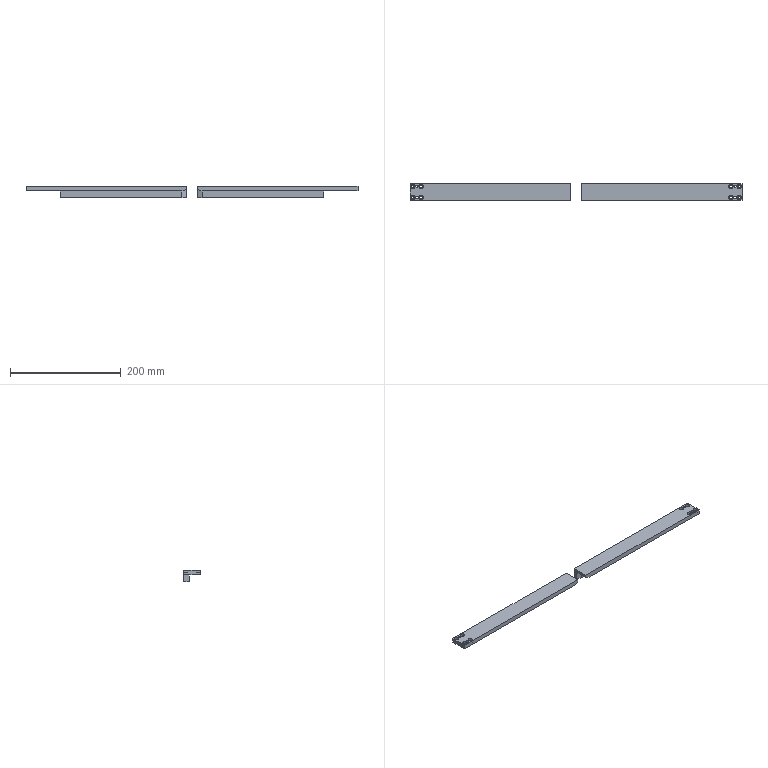NC program | NX | posted with a generic post | part box 600 x 30 x 20 mm
Lines 2675 to 3385 of 3385:
(ZLEVEL_PROFILE_COPY_1_COPY_COPY_COPY_COPY_2_COPY_1 , TOOL : D6A45)
N5306 T02 M6
N5308 G54
N5310 G17 G0 G90 X126.439 Y11.149 S7000 M3
N5312 G43 Z30. H2
N5314 Z-1.
N5316 G94 G1 X125.52 Y12.741 F1000.
N5318 G3 X125. Y13.041 R0.6
N5320 X121.959 Y10. R3.041
N5322 X125. Y13.041 R-3.041
N5324 X124.48 Y12.741 R0.6
N5326 G1 X123.561 Y11.149
N5328 G0 Z30.
N5330 X141.439
N5332 Z-1.
N5334 G1 X140.52 Y12.741
N5336 G3 X140. Y13.041 R0.6
N5338 X136.959 Y10. R3.041
N5340 X140. Y13.041 R-3.041
N5342 X139.48 Y12.741 R0.6
N5344 G1 X138.561 Y11.149
N5346 G0 Z30.
N5348 X133.541 Y-10.5
N5350 Z1.
N5352 G1 Z-1.
N5354 Y-9.5
N5356 G3 X132.5 Y-8.459 R1.041
N5358 X131.459 Y-9.5 R1.041
N5360 G1 Y-10.5
N5362 G3 X132.5 Y-11.541 R1.041
N5364 X133.541 Y-10.5 R1.041
N5366 X133.241 Y-9.98 R0.6
N5368 G0 Z30.
N5370 X123.561 Y-11.149
N5372 Z-1.
N5374 G1 X124.48 Y-12.741
N5376 G3 X125. Y-13.041 R0.6
N5378 X128.041 Y-10. R3.041
N5380 X125. Y-13.041 R-3.041
N5382 X125.52 Y-12.741 R0.6
N5384 G1 X126.439 Y-11.149
N5386 G0 Z30.
N5388 X138.561
N5390 Z-1.
N5392 G1 X139.48 Y-12.741
N5394 G3 X140. Y-13.041 R0.6
N5396 X143.041 Y-10. R3.041
N5398 X140. Y-13.041 R-3.041
N5400 X140.52 Y-12.741 R0.6
N5402 G1 X141.439 Y-11.149
N5404 G0 Z30.
N5406 X132.5 Y11.041
N5408 Z1.
N5410 G1 Z-1.
N5412 G3 X131.459 Y10. R1.041
N5414 X132.5 Y11.041 R-1.041
N5416 X131.98 Y10.741 R0.6
N5418 G0 Z30.
N5420 X-145.92 Y16.95
N5422 Z-1.
N5424 G1 X-145.521 Y16.259
N5426 G3 X-145.001 Y15.959 R0.6
N5428 G1 X145.001
N5430 G2 X145.959 Y15.001 R0.966
N5432 G1 Y-15.001
N5434 G2 X145.001 Y-15.959 R0.966
N5436 G1 X-145.001
N5438 G2 X-145.959 Y-15.001 R0.966
N5440 G1 Y15.001
N5442 G2 X-145.001 Y15.959 R0.966
N5444 G3 X-144.484 Y16.263 R0.6
N5446 G1 X-143.976 Y17.159
N5448 G0 Z30.
N5450 M5
(COMPTOOL10_COPY_1 , TOOL : D3)
N5452 T20 M6
N5454 G54
N5456 G17 G0 G90 X132.456 Y10.143 S7000 M3
N5458 G43 Z30. H20
N5460 Z-0.5
N5462 G94 G1 Z-1. F1000.
N5464 G41 X132.384 Y10.38 D20
N5466 G3 X132.119 Y10.239 R0.3
N5468 G1 X132.116 Y10.235 F850.
N5470 G3 X132.255 Y10.378 R-0.45
N5472 G1 X132.197 Y10.346
N5474 X132.15 Y10.298
N5476 X132.119 Y10.239
N5478 X132.098 Y10.185 Z-1.028
N5480 X132.078 Y10.131 Z-1.056
N5482 X132.063 Y10.075 Z-1.083
N5484 X132.058 Y10.016 Z-1.111
N5486 X132.06 Y9.958 Z-1.139
N5488 X132.068 Y9.9 Z-1.167
N5490 X132.085 Y9.845 Z-1.194
N5492 X132.102 Y9.79 Z-1.222
N5494 X132.138 Y9.744 Z-1.25
N5496 X132.175 Y9.699 Z-1.278
N5498 X132.218 Y9.66 Z-1.306
N5500 X132.265 Y9.625 Z-1.333
N5502 X132.316 Y9.598 Z-1.361
N5504 X132.37 Y9.577 Z-1.389
N5506 X132.426 Y9.564 Z-1.417
N5508 X132.484 Y9.558 Z-1.444
N5510 X132.542 Y9.56 Z-1.472
N5512 X132.599 Y9.568 Z-1.5
N5514 X132.654 Y9.585 Z-1.528
N5516 X132.707 Y9.609 Z-1.556
N5518 X132.757 Y9.64 Z-1.583
N5520 X132.801 Y9.676 Z-1.611
N5522 X132.84 Y9.718 Z-1.639
N5524 X132.875 Y9.765 Z-1.667
N5526 X132.902 Y9.816 Z-1.694
N5528 X132.923 Y9.87 Z-1.722
N5530 X132.936 Y9.926 Z-1.75
N5532 X132.942 Y9.984 Z-1.778
N5534 X132.94 Y10.042 Z-1.806
N5536 X132.932 Y10.099 Z-1.833
N5538 X132.915 Y10.154 Z-1.861
N5540 X132.891 Y10.207 Z-1.889
N5542 X132.86 Y10.257 Z-1.917
N5544 X132.824 Y10.302 Z-1.944
N5546 X132.781 Y10.341 Z-1.972
N5548 X132.739 Y10.381 Z-2.
N5550 X132.735 Y10.384
N5552 G3 X132.255 Y10.378 R0.45
N5554 G1 X132.197 Y10.346
N5556 X132.15 Y10.298
N5558 X132.119 Y10.239
N5560 X132.098 Y10.185 Z-2.028
N5562 X132.078 Y10.131 Z-2.056
N5564 X132.063 Y10.075 Z-2.083
N5566 X132.058 Y10.016 Z-2.111
N5568 X132.06 Y9.958 Z-2.139
N5570 X132.068 Y9.9 Z-2.167
N5572 X132.085 Y9.845 Z-2.194
N5574 X132.102 Y9.79 Z-2.222
N5576 X132.139 Y9.744 Z-2.25
N5578 X132.175 Y9.699 Z-2.278
N5580 X132.218 Y9.66 Z-2.306
N5582 X132.265 Y9.625 Z-2.333
N5584 X132.316 Y9.598 Z-2.361
N5586 X132.37 Y9.577 Z-2.389
N5588 X132.426 Y9.564 Z-2.417
N5590 X132.484 Y9.558 Z-2.444
N5592 X132.542 Y9.56 Z-2.472
N5594 X132.599 Y9.568 Z-2.5
N5596 X132.654 Y9.585 Z-2.528
N5598 X132.707 Y9.609 Z-2.556
N5600 X132.757 Y9.64 Z-2.583
N5602 X132.801 Y9.676 Z-2.611
N5604 X132.84 Y9.718 Z-2.639
N5606 X132.875 Y9.765 Z-2.667
N5608 X132.902 Y9.816 Z-2.694
N5610 X132.923 Y9.87 Z-2.722
N5612 X132.937 Y9.925 Z-2.75
N5614 X132.942 Y9.984 Z-2.778
N5616 X132.94 Y10.042 Z-2.806
N5618 X132.932 Y10.099 Z-2.833
N5620 X132.915 Y10.154 Z-2.861
N5622 X132.891 Y10.207 Z-2.889
N5624 X132.86 Y10.257 Z-2.917
N5626 X132.824 Y10.302 Z-2.944
N5628 X132.781 Y10.341 Z-2.972
N5630 X132.739 Y10.381 Z-3.
N5632 X132.735 Y10.384
N5634 G3 X132.255 Y10.378 R0.45
N5636 G1 X132.197 Y10.346
N5638 X132.15 Y10.298
N5640 X132.119 Y10.239
N5642 X132.098 Y10.185 Z-3.028
N5644 X132.078 Y10.131 Z-3.056
N5646 X132.063 Y10.075 Z-3.083
N5648 X132.058 Y10.016 Z-3.111
N5650 X132.06 Y9.958 Z-3.139
N5652 X132.068 Y9.9 Z-3.167
N5654 X132.085 Y9.845 Z-3.194
N5656 X132.102 Y9.79 Z-3.222
N5658 X132.139 Y9.744 Z-3.25
N5660 X132.175 Y9.699 Z-3.278
N5662 X132.218 Y9.66 Z-3.306
N5664 X132.265 Y9.625 Z-3.333
N5666 X132.316 Y9.598 Z-3.361
N5668 X132.37 Y9.577 Z-3.389
N5670 X132.425 Y9.563 Z-3.417
N5672 X132.484 Y9.558 Z-3.444
N5674 X132.542 Y9.56 Z-3.472
N5676 X132.599 Y9.568 Z-3.5
N5678 X132.654 Y9.585 Z-3.528
N5680 X132.707 Y9.609 Z-3.556
N5682 X132.757 Y9.64 Z-3.583
N5684 X132.801 Y9.676 Z-3.611
N5686 X132.84 Y9.718 Z-3.639
N5688 X132.875 Y9.765 Z-3.667
N5690 X132.902 Y9.816 Z-3.694
N5692 X132.923 Y9.87 Z-3.722
N5694 X132.937 Y9.925 Z-3.75
N5696 X132.942 Y9.984 Z-3.778
N5698 X132.94 Y10.042 Z-3.806
N5700 X132.932 Y10.099 Z-3.833
N5702 X132.915 Y10.154 Z-3.861
N5704 X132.891 Y10.207 Z-3.889
N5706 X132.86 Y10.257 Z-3.917
N5708 X132.824 Y10.302 Z-3.944
N5710 X132.781 Y10.341 Z-3.972
N5712 X132.739 Y10.381 Z-4.
N5714 X132.735 Y10.384
N5716 G3 X132.255 Y10.378 R0.45
N5718 G1 X132.197 Y10.346
N5720 X132.15 Y10.298
N5722 X132.119 Y10.239
N5724 X132.098 Y10.185 Z-4.028
N5726 X132.078 Y10.131 Z-4.056
N5728 X132.063 Y10.075 Z-4.083
N5730 X132.058 Y10.016 Z-4.111
N5732 X132.06 Y9.958 Z-4.139
N5734 X132.068 Y9.9 Z-4.167
N5736 X132.085 Y9.845 Z-4.194
N5738 X132.102 Y9.79 Z-4.222
N5740 X132.139 Y9.744 Z-4.25
N5742 X132.175 Y9.699 Z-4.278
N5744 X132.218 Y9.66 Z-4.306
N5746 X132.265 Y9.625 Z-4.333
N5748 X132.316 Y9.598 Z-4.361
N5750 X132.37 Y9.577 Z-4.389
N5752 X132.425 Y9.563 Z-4.417
N5754 X132.484 Y9.558 Z-4.444
N5756 X132.542 Y9.56 Z-4.472
N5758 X132.599 Y9.568 Z-4.5
N5760 X132.654 Y9.585 Z-4.528
N5762 X132.707 Y9.609 Z-4.556
N5764 X132.757 Y9.64 Z-4.583
N5766 X132.801 Y9.676 Z-4.611
N5768 X132.84 Y9.718 Z-4.639
N5770 X132.875 Y9.765 Z-4.667
N5772 X132.902 Y9.816 Z-4.694
N5774 X132.923 Y9.87 Z-4.722
N5776 X132.937 Y9.925 Z-4.75
N5778 X132.942 Y9.984 Z-4.778
N5780 X132.94 Y10.042 Z-4.806
N5782 X132.932 Y10.099 Z-4.833
N5784 X132.915 Y10.154 Z-4.861
N5786 X132.891 Y10.207 Z-4.889
N5788 X132.86 Y10.257 Z-4.917
N5790 X132.824 Y10.302 Z-4.944
N5792 X132.781 Y10.341 Z-4.972
N5794 X132.739 Y10.381 Z-5.
N5796 X132.735 Y10.384
N5798 G3 X132.255 Y10.378 R0.45
N5800 G1 X132.197 Y10.346
N5802 X132.15 Y10.298
N5804 X132.119 Y10.239
N5806 X132.098 Y10.185 Z-5.028
N5808 X132.078 Y10.131 Z-5.056
N5810 X132.063 Y10.075 Z-5.083
N5812 X132.058 Y10.016 Z-5.111
N5814 X132.06 Y9.958 Z-5.139
N5816 X132.068 Y9.9 Z-5.167
N5818 X132.085 Y9.845 Z-5.194
N5820 X132.102 Y9.79 Z-5.222
N5822 X132.139 Y9.744 Z-5.25
N5824 X132.175 Y9.699 Z-5.278
N5826 X132.218 Y9.66 Z-5.306
N5828 X132.265 Y9.625 Z-5.333
N5830 X132.316 Y9.598 Z-5.361
N5832 X132.37 Y9.577 Z-5.389
N5834 X132.425 Y9.563 Z-5.417
N5836 X132.484 Y9.558 Z-5.444
N5838 X132.542 Y9.56 Z-5.472
N5840 X132.599 Y9.568 Z-5.5
N5842 X132.654 Y9.585 Z-5.528
N5844 X132.707 Y9.609 Z-5.556
N5846 X132.757 Y9.64 Z-5.583
N5848 X132.801 Y9.676 Z-5.611
N5850 X132.84 Y9.718 Z-5.639
N5852 X132.875 Y9.765 Z-5.667
N5854 X132.902 Y9.816 Z-5.694
N5856 X132.923 Y9.87 Z-5.722
N5858 X132.937 Y9.925 Z-5.75
N5860 X132.942 Y9.984 Z-5.778
N5862 X132.94 Y10.042 Z-5.806
N5864 X132.932 Y10.099 Z-5.833
N5866 X132.915 Y10.154 Z-5.861
N5868 X132.891 Y10.207 Z-5.889
N5870 X132.86 Y10.257 Z-5.917
N5872 X132.824 Y10.302 Z-5.944
N5874 X132.781 Y10.341 Z-5.972
N5876 X132.739 Y10.381 Z-6.
N5878 X132.735 Y10.384
N5880 G3 X132.255 Y10.378 R0.45
N5882 G1 X132.197 Y10.346
N5884 X132.15 Y10.298
N5886 X132.119 Y10.239
N5888 X132.099 Y10.185 Z-6.028
N5890 X132.078 Y10.131 Z-6.056
N5892 X132.063 Y10.075 Z-6.083
N5894 X132.058 Y10.016 Z-6.111
N5896 X132.06 Y9.958 Z-6.139
N5898 X132.068 Y9.9 Z-6.167
N5900 X132.085 Y9.845 Z-6.194
N5902 X132.102 Y9.79 Z-6.222
N5904 X132.139 Y9.744 Z-6.25
N5906 X132.175 Y9.699 Z-6.278
N5908 X132.218 Y9.66 Z-6.306
N5910 X132.265 Y9.625 Z-6.333
N5912 X132.316 Y9.598 Z-6.361
N5914 X132.37 Y9.577 Z-6.389
N5916 X132.425 Y9.563 Z-6.417
N5918 X132.484 Y9.558 Z-6.444
N5920 X132.542 Y9.56 Z-6.472
N5922 X132.599 Y9.568 Z-6.5
N5924 X132.654 Y9.585 Z-6.528
N5926 X132.707 Y9.609 Z-6.556
N5928 X132.757 Y9.639 Z-6.583
N5930 X132.801 Y9.676 Z-6.611
N5932 X132.84 Y9.718 Z-6.639
N5934 X132.874 Y9.765 Z-6.667
N5936 X132.902 Y9.816 Z-6.694
N5938 X132.923 Y9.87 Z-6.722
N5940 X132.937 Y9.925 Z-6.75
N5942 X132.942 Y9.984 Z-6.778
N5944 X132.94 Y10.042 Z-6.806
N5946 X132.932 Y10.099 Z-6.833
N5948 X132.915 Y10.154 Z-6.861
N5950 X132.891 Y10.207 Z-6.889
N5952 X132.86 Y10.257 Z-6.917
N5954 X132.824 Y10.302 Z-6.944
N5956 X132.781 Y10.341 Z-6.972
N5958 X132.739 Y10.381 Z-7.
N5960 X132.735 Y10.384
N5962 G3 X132.255 Y10.378 R0.45
N5964 G1 X132.197 Y10.346
N5966 X132.15 Y10.298
N5968 X132.119 Y10.239
N5970 X132.099 Y10.185 Z-7.028
N5972 X132.078 Y10.131 Z-7.056
N5974 X132.063 Y10.075 Z-7.083
N5976 X132.058 Y10.016 Z-7.111
N5978 X132.06 Y9.958 Z-7.139
N5980 X132.068 Y9.9 Z-7.167
N5982 X132.085 Y9.845 Z-7.194
N5984 X132.102 Y9.79 Z-7.222
N5986 X132.139 Y9.745 Z-7.25
N5988 X132.175 Y9.699 Z-7.278
N5990 X132.218 Y9.66 Z-7.306
N5992 X132.265 Y9.625 Z-7.333
N5994 X132.316 Y9.598 Z-7.361
N5996 X132.37 Y9.577 Z-7.389
N5998 X132.425 Y9.563 Z-7.417
N6000 X132.484 Y9.558 Z-7.444
N6002 X132.542 Y9.56 Z-7.472
N6004 X132.599 Y9.568 Z-7.5
N6006 X132.654 Y9.585 Z-7.528
N6008 X132.707 Y9.609 Z-7.556
N6010 X132.757 Y9.639 Z-7.583
N6012 X132.801 Y9.676 Z-7.611
N6014 X132.84 Y9.718 Z-7.639
N6016 X132.874 Y9.765 Z-7.667
N6018 X132.902 Y9.816 Z-7.694
N6020 X132.923 Y9.87 Z-7.722
N6022 X132.937 Y9.925 Z-7.75
N6024 X132.942 Y9.984 Z-7.778
N6026 X132.94 Y10.042 Z-7.806
N6028 X132.932 Y10.099 Z-7.833
N6030 X132.915 Y10.154 Z-7.861
N6032 X132.891 Y10.207 Z-7.889
N6034 X132.86 Y10.257 Z-7.917
N6036 X132.824 Y10.302 Z-7.944
N6038 X132.781 Y10.341 Z-7.972
N6040 X132.739 Y10.381 Z-8.
N6042 X132.735 Y10.384
N6044 G3 X132.255 Y10.378 R0.45
N6046 X132.116 Y10.235 R0.45
N6048 X132.878 Y10.245 R-0.45
N6050 G1 X132.846 Y10.303
N6052 X132.798 Y10.35
N6054 X132.739 Y10.381
N6056 G3 X132.439 Y10.392 R0.3
N6058 G40
N6060 G1 X132.477 Y10.148
N6062 Z-7.5
N6064 G0 Z30.
N6066 X132.444 Y-9.619
N6068 Z-0.5
N6070 G1 Z-1. F1000.
N6072 G41 X132.35 Y-9.654
N6074 X132.2 Y-9.74
N6076 G3 X132.05 Y-10. R0.3
N6078 G1 Y-10.5 F850.
N6080 G3 X132.5 Y-10.95 R0.45
N6082 X132.95 Y-10.5 R0.45
N6084 G1 Y-9.5
N6086 G3 X132.5 Y-9.05 R0.45
N6088 X132.05 Y-9.5 R0.45
N6090 G1 Y-10.
N6092 Y-10.362 Z-1.1
N6094 X132.054 Y-10.483 Z-1.133
N6096 X132.06 Y-10.542 Z-1.15
N6098 X132.062 Y-10.602 Z-1.167
N6100 X132.079 Y-10.659 Z-1.183
N6102 X132.111 Y-10.711 Z-1.2
N6104 X132.143 Y-10.762 Z-1.217
N6106 X132.181 Y-10.807 Z-1.233
N6108 X132.225 Y-10.846 Z-1.25
N6110 X132.274 Y-10.88 Z-1.267
N6112 X132.327 Y-10.909 Z-1.283
N6114 X132.383 Y-10.926 Z-1.3
N6116 X132.441 Y-10.938 Z-1.317
N6118 X132.5 Y-10.944 Z-1.333
N6120 X132.559 Y-10.938 Z-1.35
N6122 X132.617 Y-10.926 Z-1.367
N6124 X132.673 Y-10.909 Z-1.383
N6126 X132.726 Y-10.88 Z-1.4
N6128 X132.775 Y-10.846 Z-1.417
N6130 X132.819 Y-10.807 Z-1.433
N6132 X132.857 Y-10.762 Z-1.45
N6134 X132.889 Y-10.711 Z-1.467
N6136 X132.914 Y-10.657 Z-1.483
N6138 X132.931 Y-10.601 Z-1.5
N6140 X132.94 Y-10.542 Z-1.517
N6142 X132.946 Y-10.483 Z-1.533
N6144 X132.95 Y-10.362 Z-1.567
N6146 Y-9.638 Z-1.767
N6148 X132.946 Y-9.517 Z-1.8
N6150 X132.94 Y-9.458 Z-1.817
N6152 X132.931 Y-9.399 Z-1.833
N6154 X132.914 Y-9.343 Z-1.85
N6156 X132.889 Y-9.289 Z-1.867
N6158 X132.857 Y-9.238 Z-1.883
N6160 X132.819 Y-9.193 Z-1.9
N6162 X132.775 Y-9.154 Z-1.917
N6164 X132.726 Y-9.12 Z-1.933
N6166 X132.673 Y-9.091 Z-1.95
N6168 X132.616 Y-9.074 Z-1.967
N6170 X132.558 Y-9.062 Z-1.983
N6172 X132.5 Y-9.05 Z-2.
N6174 G3 X132.05 Y-9.5 R0.45
N6176 G1 Y-10.
N6178 Y-10.362 Z-2.1
N6180 X132.054 Y-10.483 Z-2.133
N6182 X132.06 Y-10.542 Z-2.15
N6184 X132.062 Y-10.602 Z-2.167
N6186 X132.079 Y-10.659 Z-2.183
N6188 X132.111 Y-10.711 Z-2.2
N6190 X132.143 Y-10.762 Z-2.217
N6192 X132.181 Y-10.807 Z-2.233
N6194 X132.225 Y-10.846 Z-2.25
N6196 X132.274 Y-10.88 Z-2.267
N6198 X132.327 Y-10.909 Z-2.283
N6200 X132.383 Y-10.926 Z-2.3
N6202 X132.441 Y-10.938 Z-2.317
N6204 X132.5 Y-10.944 Z-2.333
N6206 X132.559 Y-10.938 Z-2.35
N6208 X132.617 Y-10.926 Z-2.367
N6210 X132.673 Y-10.909 Z-2.383
N6212 X132.726 Y-10.88 Z-2.4
N6214 X132.775 Y-10.846 Z-2.417
N6216 X132.819 Y-10.807 Z-2.433
N6218 X132.857 Y-10.762 Z-2.45
N6220 X132.889 Y-10.711 Z-2.467
N6222 X132.914 Y-10.657 Z-2.483
N6224 X132.931 Y-10.601 Z-2.5
N6226 X132.94 Y-10.542 Z-2.517
N6228 X132.946 Y-10.483 Z-2.533
N6230 X132.95 Y-10.362 Z-2.567
N6232 Y-9.638 Z-2.767
N6234 X132.946 Y-9.517 Z-2.8
N6236 X132.94 Y-9.458 Z-2.817
N6238 X132.931 Y-9.399 Z-2.833
N6240 X132.914 Y-9.343 Z-2.85
N6242 X132.889 Y-9.289 Z-2.867
N6244 X132.857 Y-9.238 Z-2.883
N6246 X132.819 Y-9.193 Z-2.9
N6248 X132.775 Y-9.154 Z-2.917
N6250 X132.726 Y-9.12 Z-2.933
N6252 X132.673 Y-9.091 Z-2.95
N6254 X132.616 Y-9.074 Z-2.967
N6256 X132.558 Y-9.062 Z-2.983
N6258 X132.5 Y-9.05 Z-3.
N6260 G3 X132.05 Y-9.5 R0.45
N6262 G1 Y-10.
N6264 Y-10.362 Z-3.1
N6266 X132.054 Y-10.483 Z-3.133
N6268 X132.06 Y-10.542 Z-3.15
N6270 X132.062 Y-10.602 Z-3.167
N6272 X132.079 Y-10.659 Z-3.183
N6274 X132.111 Y-10.711 Z-3.2
N6276 X132.143 Y-10.762 Z-3.217
N6278 X132.181 Y-10.807 Z-3.233
N6280 X132.225 Y-10.846 Z-3.25
N6282 X132.274 Y-10.88 Z-3.267
N6284 X132.327 Y-10.909 Z-3.283
N6286 X132.383 Y-10.926 Z-3.3
N6288 X132.441 Y-10.938 Z-3.317
N6290 X132.5 Y-10.944 Z-3.333
N6292 X132.559 Y-10.938 Z-3.35
N6294 X132.617 Y-10.926 Z-3.367
N6296 X132.673 Y-10.909 Z-3.383
N6298 X132.726 Y-10.88 Z-3.4
N6300 X132.775 Y-10.846 Z-3.417
N6302 X132.819 Y-10.807 Z-3.433
N6304 X132.857 Y-10.762 Z-3.45
N6306 X132.889 Y-10.711 Z-3.467
N6308 X132.914 Y-10.657 Z-3.483
N6310 X132.931 Y-10.601 Z-3.5
N6312 X132.94 Y-10.542 Z-3.517
N6314 X132.946 Y-10.483 Z-3.533
N6316 X132.95 Y-10.362 Z-3.567
N6318 Y-9.638 Z-3.767
N6320 X132.946 Y-9.517 Z-3.8
N6322 X132.94 Y-9.458 Z-3.817
N6324 X132.931 Y-9.399 Z-3.833
N6326 X132.914 Y-9.343 Z-3.85
N6328 X132.888 Y-9.289 Z-3.867
N6330 X132.857 Y-9.238 Z-3.883
N6332 X132.819 Y-9.193 Z-3.9
N6334 X132.775 Y-9.154 Z-3.917
N6336 X132.726 Y-9.12 Z-3.933
N6338 X132.673 Y-9.091 Z-3.95
N6340 X132.616 Y-9.074 Z-3.967
N6342 X132.558 Y-9.062 Z-3.983
N6344 X132.5 Y-9.05 Z-4.
N6346 G3 X132.05 Y-9.5 R0.45
N6348 G1 Y-10.
N6350 Y-10.362 Z-4.1
N6352 X132.054 Y-10.483 Z-4.133
N6354 X132.06 Y-10.542 Z-4.15
N6356 X132.062 Y-10.602 Z-4.167
N6358 X132.079 Y-10.659 Z-4.183
N6360 X132.112 Y-10.711 Z-4.2
N6362 X132.143 Y-10.762 Z-4.217
N6364 X132.181 Y-10.807 Z-4.233
N6366 X132.225 Y-10.846 Z-4.25
N6368 X132.274 Y-10.88 Z-4.267
N6370 X132.327 Y-10.909 Z-4.283
N6372 X132.383 Y-10.926 Z-4.3
N6374 X132.441 Y-10.938 Z-4.317
N6376 X132.5 Y-10.944 Z-4.333
N6378 X132.559 Y-10.938 Z-4.35
N6380 X132.617 Y-10.926 Z-4.367
N6382 X132.673 Y-10.909 Z-4.383
N6384 X132.726 Y-10.88 Z-4.4
N6386 X132.775 Y-10.846 Z-4.417
N6388 X132.819 Y-10.807 Z-4.433
N6390 X132.857 Y-10.762 Z-4.45
N6392 X132.888 Y-10.711 Z-4.467
N6394 X132.914 Y-10.657 Z-4.483
N6396 X132.931 Y-10.601 Z-4.5
N6398 X132.94 Y-10.542 Z-4.517
N6400 X132.946 Y-10.483 Z-4.533
N6402 X132.95 Y-10.362 Z-4.567
N6404 Y-9.638 Z-4.767
N6406 X132.946 Y-9.517 Z-4.8
N6408 X132.94 Y-9.458 Z-4.817
N6410 X132.931 Y-9.399 Z-4.833
N6412 X132.914 Y-9.343 Z-4.85
N6414 X132.888 Y-9.289 Z-4.867
N6416 X132.857 Y-9.238 Z-4.883
N6418 X132.819 Y-9.193 Z-4.9
N6420 X132.775 Y-9.154 Z-4.917
N6422 X132.726 Y-9.12 Z-4.933
N6424 X132.673 Y-9.091 Z-4.95
N6426 X132.616 Y-9.074 Z-4.967
N6428 X132.558 Y-9.062 Z-4.983
N6430 X132.5 Y-9.05 Z-5.
N6432 G3 X132.05 Y-9.5 R0.45
N6434 G1 Y-10.
N6436 Y-10.362 Z-5.1
N6438 X132.054 Y-10.483 Z-5.133
N6440 X132.06 Y-10.542 Z-5.15
N6442 X132.062 Y-10.602 Z-5.167
N6444 X132.079 Y-10.659 Z-5.183
N6446 X132.112 Y-10.711 Z-5.2
N6448 X132.143 Y-10.762 Z-5.217
N6450 X132.181 Y-10.807 Z-5.233
N6452 X132.225 Y-10.846 Z-5.25
N6454 X132.274 Y-10.88 Z-5.267
N6456 X132.327 Y-10.909 Z-5.283
N6458 X132.383 Y-10.926 Z-5.3
N6460 X132.441 Y-10.938 Z-5.317
N6462 X132.5 Y-10.944 Z-5.333
N6464 X132.559 Y-10.938 Z-5.35
N6466 X132.617 Y-10.926 Z-5.367
N6468 X132.673 Y-10.909 Z-5.383
N6470 X132.726 Y-10.88 Z-5.4
N6472 X132.775 Y-10.846 Z-5.417
N6474 X132.819 Y-10.807 Z-5.433
N6476 X132.857 Y-10.762 Z-5.45
N6478 X132.888 Y-10.711 Z-5.467
N6480 X132.914 Y-10.657 Z-5.483
N6482 X132.931 Y-10.601 Z-5.5
N6484 X132.94 Y-10.542 Z-5.517
N6486 X132.946 Y-10.483 Z-5.533
N6488 X132.95 Y-10.362 Z-5.567
N6490 Y-9.638 Z-5.767
N6492 X132.946 Y-9.517 Z-5.8
N6494 X132.94 Y-9.458 Z-5.817
N6496 X132.931 Y-9.399 Z-5.833
N6498 X132.914 Y-9.343 Z-5.85
N6500 X132.888 Y-9.289 Z-5.867
N6502 X132.857 Y-9.238 Z-5.883
N6504 X132.819 Y-9.193 Z-5.9
N6506 X132.775 Y-9.154 Z-5.917
N6508 X132.726 Y-9.12 Z-5.933
N6510 X132.673 Y-9.091 Z-5.95
N6512 X132.616 Y-9.074 Z-5.967
N6514 X132.558 Y-9.062 Z-5.983
N6516 X132.5 Y-9.05 Z-6.
N6518 G3 X132.05 Y-9.5 R0.45
N6520 G1 Y-10.
N6522 Y-10.362 Z-6.1
N6524 X132.054 Y-10.483 Z-6.133
N6526 X132.06 Y-10.542 Z-6.15
N6528 X132.062 Y-10.602 Z-6.167
N6530 X132.079 Y-10.659 Z-6.183
N6532 X132.112 Y-10.711 Z-6.2
N6534 X132.143 Y-10.762 Z-6.217
N6536 X132.181 Y-10.807 Z-6.233
N6538 X132.225 Y-10.846 Z-6.25
N6540 X132.274 Y-10.88 Z-6.267
N6542 X132.327 Y-10.909 Z-6.283
N6544 X132.383 Y-10.926 Z-6.3
N6546 X132.441 Y-10.938 Z-6.317
N6548 X132.5 Y-10.944 Z-6.333
N6550 X132.559 Y-10.938 Z-6.35
N6552 X132.617 Y-10.926 Z-6.367
N6554 X132.673 Y-10.909 Z-6.383
N6556 X132.726 Y-10.88 Z-6.4
N6558 X132.775 Y-10.846 Z-6.417
N6560 X132.819 Y-10.807 Z-6.433
N6562 X132.857 Y-10.762 Z-6.45
N6564 X132.888 Y-10.711 Z-6.467
N6566 X132.914 Y-10.657 Z-6.483
N6568 X132.931 Y-10.601 Z-6.5
N6570 X132.939 Y-10.542 Z-6.517
N6572 X132.946 Y-10.483 Z-6.533
N6574 X132.95 Y-10.362 Z-6.567
N6576 Y-9.638 Z-6.767
N6578 X132.946 Y-9.517 Z-6.8
N6580 X132.939 Y-9.458 Z-6.817
N6582 X132.931 Y-9.399 Z-6.833
N6584 X132.914 Y-9.343 Z-6.85
N6586 X132.888 Y-9.289 Z-6.867
N6588 X132.857 Y-9.238 Z-6.883
N6590 X132.819 Y-9.193 Z-6.9
N6592 X132.775 Y-9.154 Z-6.917
N6594 X132.726 Y-9.12 Z-6.933
N6596 X132.673 Y-9.091 Z-6.95
N6598 X132.616 Y-9.074 Z-6.967
N6600 X132.558 Y-9.062 Z-6.983
N6602 X132.5 Y-9.05 Z-7.
N6604 G3 X132.05 Y-9.5 R0.45
N6606 G1 Y-10.
N6608 Y-10.362 Z-7.1
N6610 X132.054 Y-10.483 Z-7.133
N6612 X132.06 Y-10.542 Z-7.15
N6614 X132.062 Y-10.602 Z-7.167
N6616 X132.079 Y-10.659 Z-7.183
N6618 X132.112 Y-10.711 Z-7.2
N6620 X132.143 Y-10.762 Z-7.217
N6622 X132.181 Y-10.807 Z-7.233
N6624 X132.225 Y-10.846 Z-7.25
N6626 X132.274 Y-10.88 Z-7.267
N6628 X132.327 Y-10.909 Z-7.283
N6630 X132.383 Y-10.926 Z-7.3
N6632 X132.441 Y-10.938 Z-7.317
N6634 X132.5 Y-10.944 Z-7.333
N6636 X132.559 Y-10.938 Z-7.35
N6638 X132.617 Y-10.926 Z-7.367
N6640 X132.673 Y-10.909 Z-7.383
N6642 X132.726 Y-10.88 Z-7.4
N6644 X132.775 Y-10.846 Z-7.417
N6646 X132.819 Y-10.807 Z-7.433
N6648 X132.857 Y-10.762 Z-7.45
N6650 X132.888 Y-10.711 Z-7.467
N6652 X132.914 Y-10.657 Z-7.483
N6654 X132.931 Y-10.601 Z-7.5
N6656 X132.939 Y-10.542 Z-7.517
N6658 X132.946 Y-10.483 Z-7.533
N6660 X132.95 Y-10.362 Z-7.567
N6662 Y-9.638 Z-7.767
N6664 X132.946 Y-9.517 Z-7.8
N6666 X132.939 Y-9.458 Z-7.817
N6668 X132.931 Y-9.399 Z-7.833
N6670 X132.914 Y-9.343 Z-7.85
N6672 X132.888 Y-9.289 Z-7.867
N6674 X132.857 Y-9.238 Z-7.883
N6676 X132.819 Y-9.193 Z-7.9
N6678 X132.775 Y-9.154 Z-7.917
N6680 X132.726 Y-9.12 Z-7.933
N6682 X132.673 Y-9.091 Z-7.95
N6684 X132.616 Y-9.074 Z-7.967
N6686 X132.558 Y-9.062 Z-7.983
N6688 X132.5 Y-9.05 Z-8.
N6690 G3 X132.05 Y-9.5 R0.45
N6692 G1 Y-10.5
N6694 G3 X132.5 Y-10.95 R0.45
N6696 X132.95 Y-10.5 R0.45
N6698 G1 Y-9.5
N6700 G3 X132.5 Y-9.05 R0.45
N6702 X132.24 Y-9.2 R0.3
N6704 G40
N6706 G1 X132.402 Y-9.387
N6708 Z-7.5
N6710 G0 Z30.
N6712 M5
N6714 M2